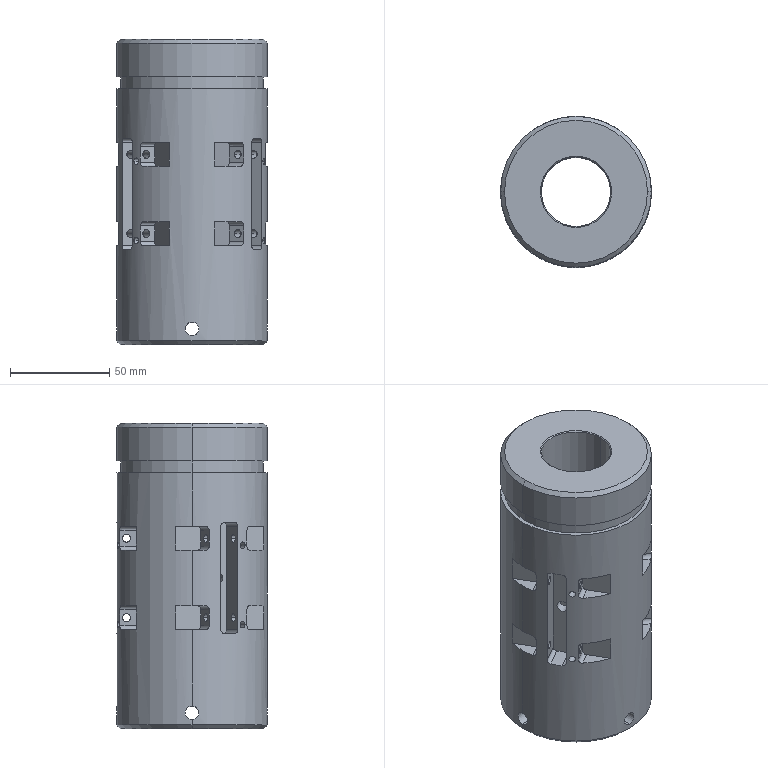Part | STEP file | 2090 Fixed material shaft | 1 solid | 184 faces | box 76 x 76 x 154 mm | volume 511727 mm3 | cylinder 94 | plane 70 | cone 20 | commonest cylinder face diameters 4 x60 3.3 x12 6.8 x8 6 x6 76 x4 35 x2